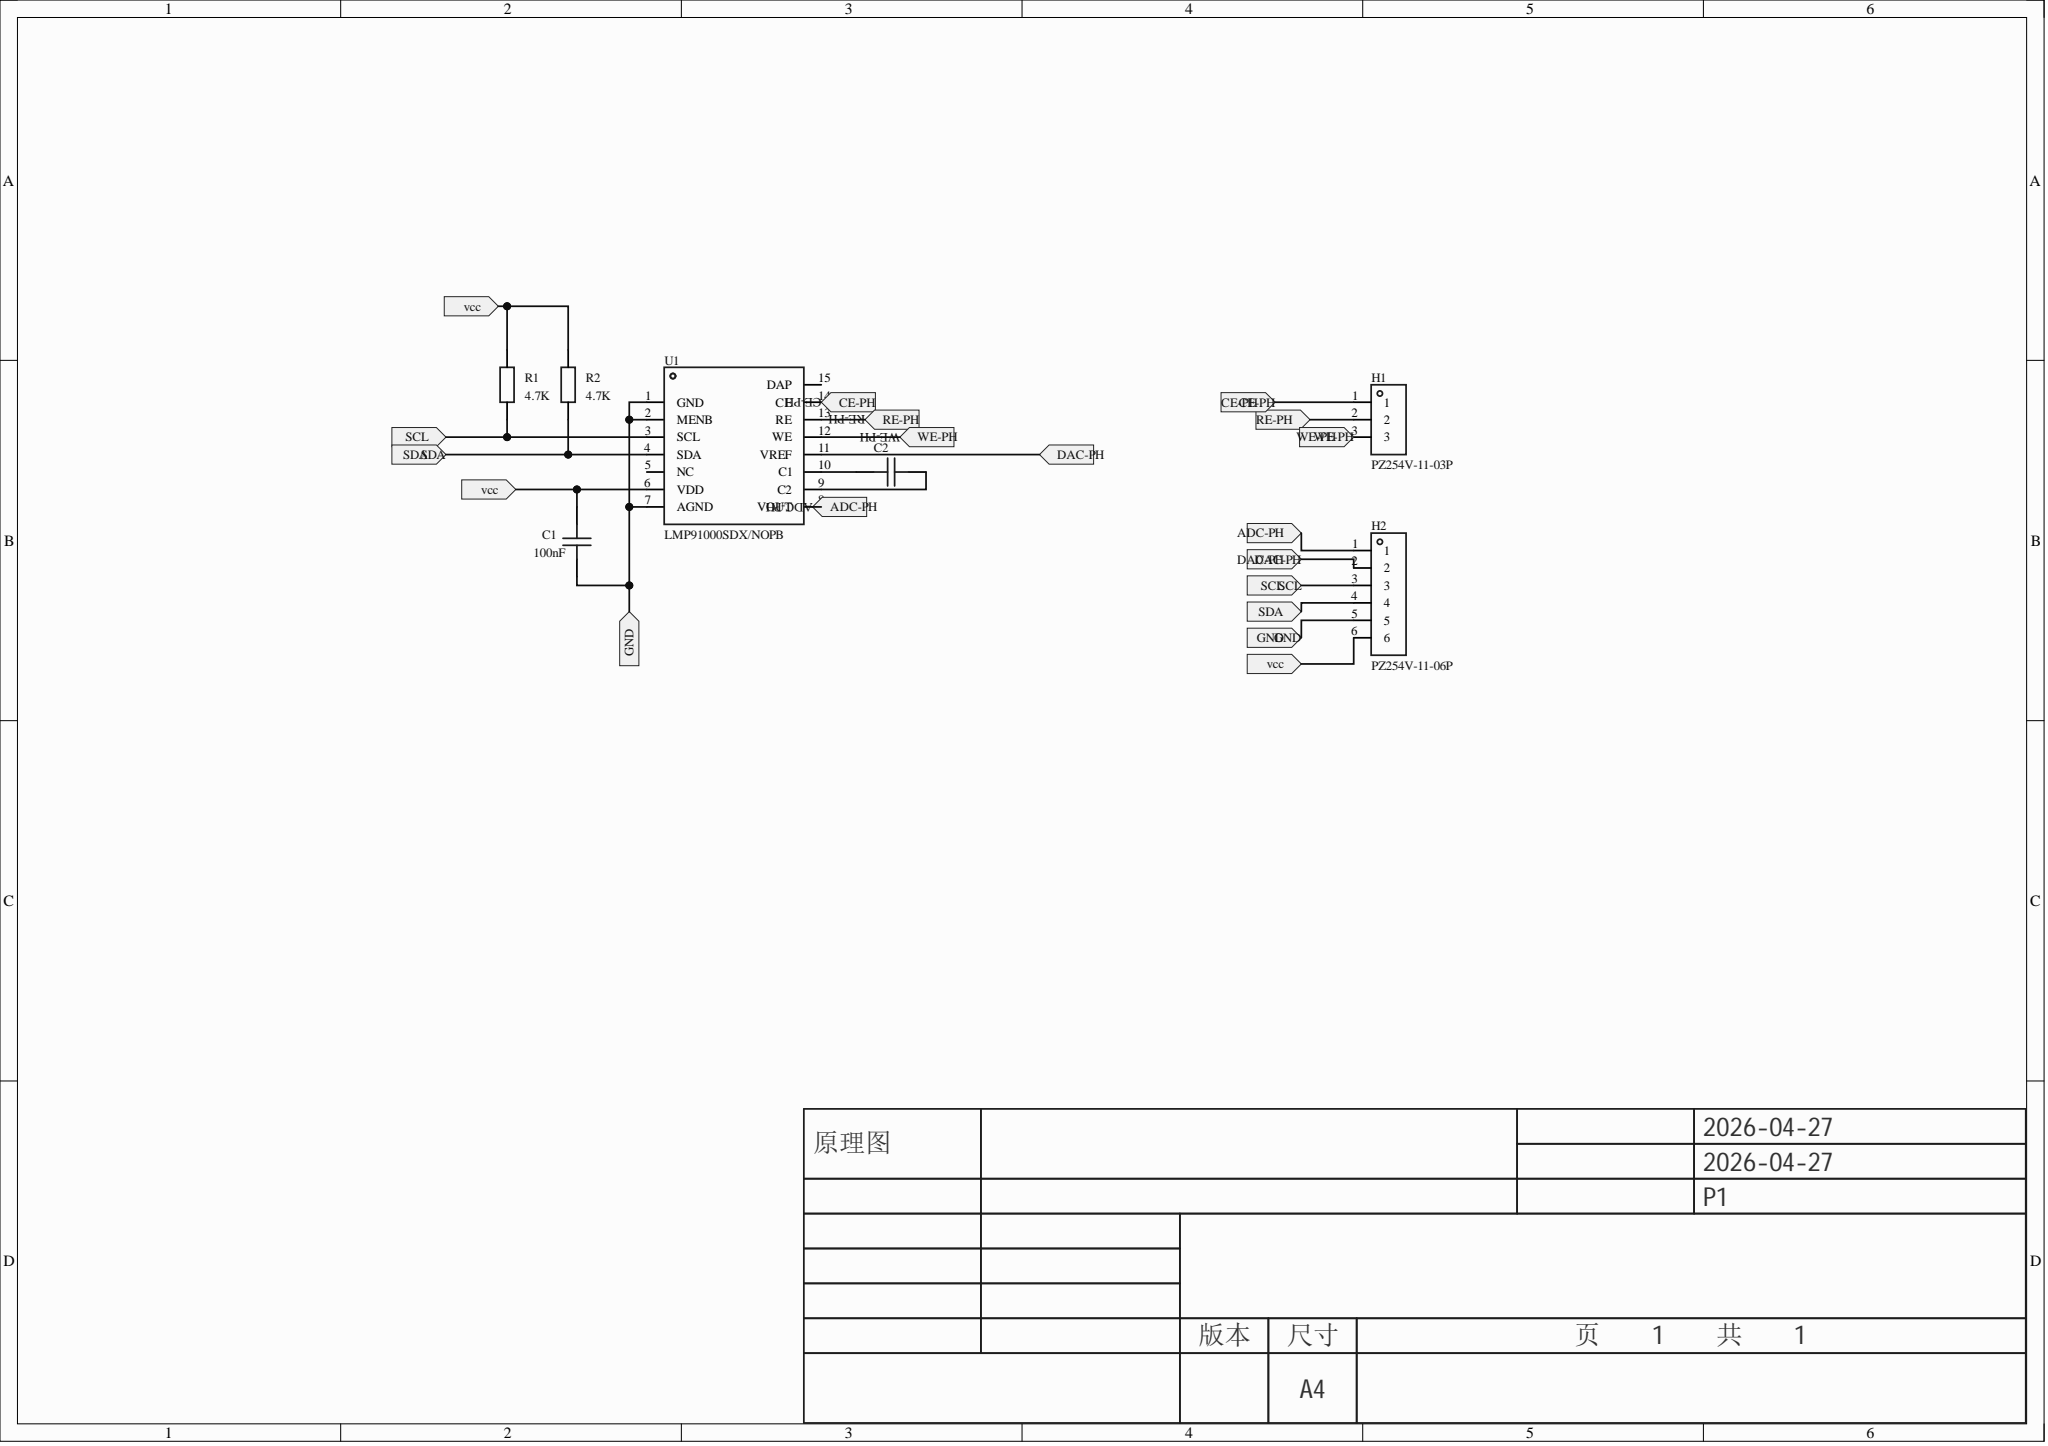Circuit board | Altium Designer | 7 parts | 11 nets
Bill of materials:
Comment,Description,Designator,Footprint,LibRef,Quantity
"100nF","","C1","C0603","CAP_0603","1"
"","","C2","C0603","CAP_0603","1"
"PZ254V-11-03P","插针结构:1x3P;间距:2.54mm;行距:-;圆针/方针:方针;安装方式:直插;排数:单排;总PIN位数:3P;额定电流:3A;额定电压:250V;配合针长度:6mm;塑高:2.5mm;端接针长度:3mm;工作温度:-40℃~+105℃;颜色:黑色;","H1","HDR-TH_3P-P2.54-V-M_PZ254V-11-03P","PZ254V-11-03P","1"
"PZ254V-11-06P","插针结构:1x6P;间距:2.54mm;行距:-;圆针/方针:方针;安装方式:直插;排数:单排;总PIN位数:6P;额定电流:3A;额定电压:250V;配合针长度:6mm;塑高:2.5mm;端接针长度:3mm;触头材质:黄铜;触头镀层:-;工作温度:-40℃~+105℃;颜色:黑色;","H2","HDR-TH_6P-P2.54-V-M","PZ254V-11-06P","1"
"4.7K","","R1, R2","R0603","Res_0603","2"
"LMP91000SDX/NOPB","工作电压:2.7V~5.25V;工作电流:-;","U1","WSON-14_L4.0-W4.0-P0.50-BL-EP-1","LMP91000SDX/NOPB","1"
Netlist (Protel format):
[
C1
C0603
100nF



]
[
C2
C0603




]
[
H1
HDR-TH_3P-P2.54-V-M_PZ254V-11-03P
PZ254V-11-03P



]
[
H2
HDR-TH_6P-P2.54-V-M
PZ254V-11-06P



]
[
R1
R0603
4.7K



]
[
R2
R0603
4.7K



]
[
U1
WSON-14_L4.0-W4.0-P0.50-BL-EP-1
LMP91000SDX/NOPB



]
(
WE-PH
H1-3
U1-12
)
(
SDA
H2-4
R2-1
U1-4
)
(
SCL
H2-3
R1-1
U1-3
)
(
RE-PH
H1-2
U1-13
)
(
NetC2_2
C2-2
U1-9
)
(
NetC2_1
C2-1
U1-10
)
(
NetC1_1
C1-1
H2-6
R1-2
R2-2
U1-6
)
(
GND
C1-2
H2-5
U1-1
U1-2
U1-7
)
(
DAC-PH
H2-2
U1-11
)
(
CE-PH
H1-1
U1-14
)
(
ADC-PH
H2-1
U1-8
)